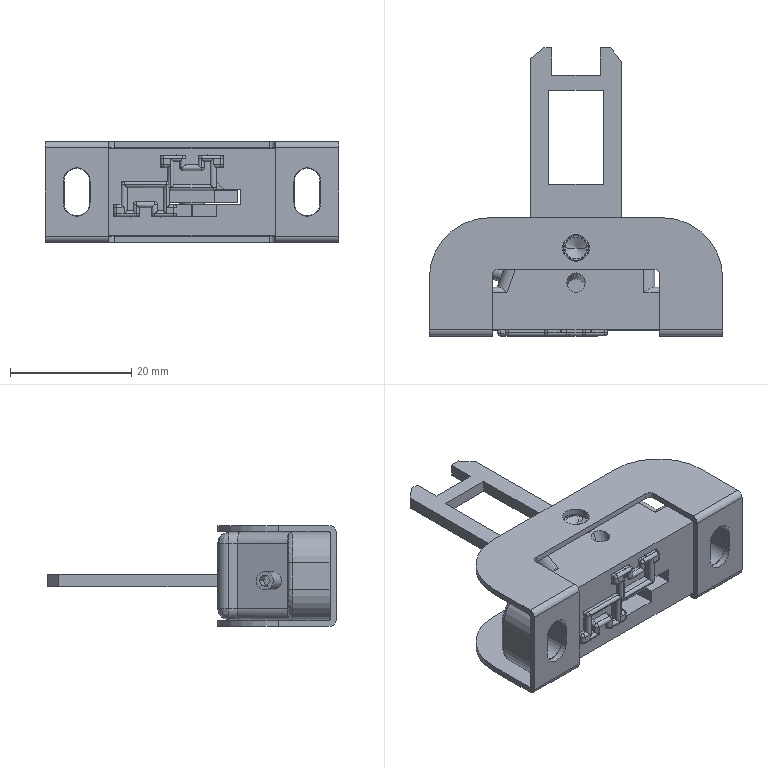Part | SolidWorks | features BaseBody 7, MoveCopyBody 1 | 7 solids | 430 faces | box 48.4 x 47.5 x 16.6 mm | volume 8438 mm3 | plane 213 | cylinder 165 | spline 48 | cone 4 | commonest cylinder face diameters 1 x88 4.2 x12 3.6 x10 2 x8 4.4 x8 1.6 x6